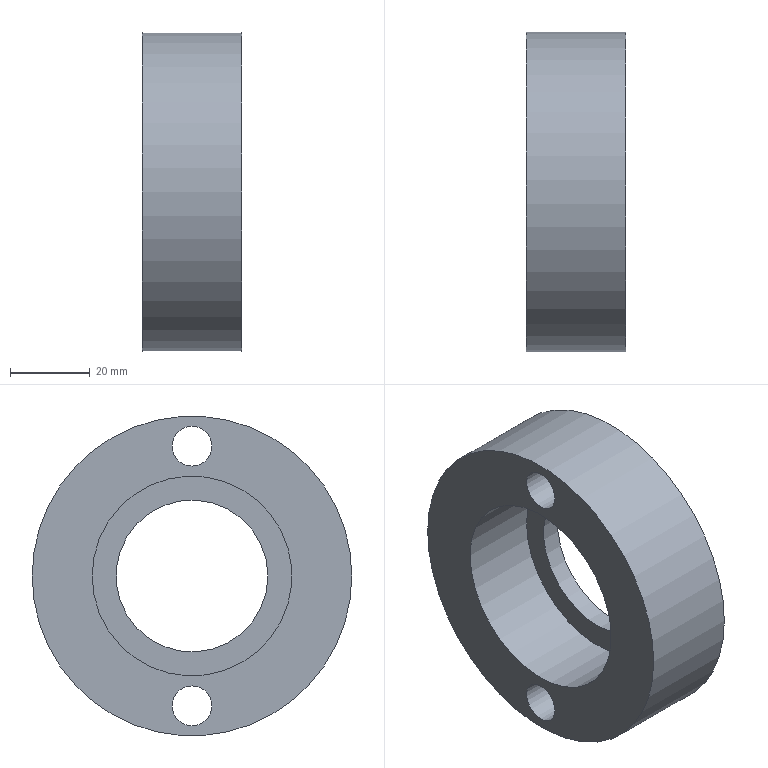Part | NX | features Hydraulic support1 2 | 1 solid | 8 faces | box 25 x 80 x 80 mm | volume 76796 mm3 | cylinder 5 | plane 3 | commonest cylinder face diameters 10 x2 38 x1 50 x1 80 x1
STEP:
#1=CARTESIAN_POINT('',(10.65,25.,0.));
#2=VERTEX_POINT('',#1);
#3=CARTESIAN_POINT('',(10.65,0.,0.));
#4=DIRECTION('',(1.,0.,0.));
#5=DIRECTION('',(0.,1.,0.));
#6=AXIS2_PLACEMENT_3D('',#3,#4,#5);
#7=CIRCLE('',#6,25.);
#8=EDGE_CURVE('',#2,#2,#7,.T.);
#9=ORIENTED_EDGE('',*,*,#8,.T.);
#10=EDGE_LOOP('',(#9));
#11=FACE_BOUND('',#10,.T.);
#12=CARTESIAN_POINT('',(-9.35,25.,0.));
#13=VERTEX_POINT('',#12);
#14=CARTESIAN_POINT('',(-9.35,0.,0.));
#15=DIRECTION('',(1.,0.,0.));
#16=DIRECTION('',(0.,1.,0.));
#17=AXIS2_PLACEMENT_3D('',#14,#15,#16);
#18=CIRCLE('',#17,25.);
#19=EDGE_CURVE('',#13,#13,#18,.F.);
#20=ORIENTED_EDGE('',*,*,#19,.T.);
#21=EDGE_LOOP('',(#20));
#22=FACE_BOUND('',#21,.T.);
#23=CARTESIAN_POINT('',(-9.35,0.,0.));
#24=DIRECTION('',(1.,0.,0.));
#25=DIRECTION('',(0.,1.,0.));
#26=AXIS2_PLACEMENT_3D('',#23,#24,#25);
#27=CYLINDRICAL_SURFACE('',#26,25.);
#28=ADVANCED_FACE('',(#11,#22),#27,.F.);
#29=CARTESIAN_POINT('',(-9.35,40.,0.));
#30=VERTEX_POINT('',#29);
#31=CARTESIAN_POINT('',(-9.35,0.,0.));
#32=DIRECTION('',(1.,0.,0.));
#33=DIRECTION('',(0.,1.,0.));
#34=AXIS2_PLACEMENT_3D('',#31,#32,#33);
#35=CIRCLE('',#34,40.);
#36=EDGE_CURVE('',#30,#30,#35,.T.);
#37=ORIENTED_EDGE('',*,*,#36,.F.);
#38=EDGE_LOOP('',(#37));
#39=FACE_BOUND('',#38,.T.);
#40=ORIENTED_EDGE('',*,*,#19,.F.);
#41=EDGE_LOOP('',(#40));
#42=FACE_BOUND('',#41,.T.);
#43=CARTESIAN_POINT('',(-9.35,0.,-37.5));
#44=VERTEX_POINT('',#43);
#45=CARTESIAN_POINT('',(-9.35,0.,-32.5));
#46=DIRECTION('',(1.,0.,0.));
#47=DIRECTION('',(0.,0.,-1.));
#48=AXIS2_PLACEMENT_3D('',#45,#46,#47);
#49=CIRCLE('',#48,5.);
#50=EDGE_CURVE('',#44,#44,#49,.T.);
#51=ORIENTED_EDGE('',*,*,#50,.T.);
#52=EDGE_LOOP('',(#51));
#53=FACE_BOUND('',#52,.T.);
#54=CARTESIAN_POINT('',(-9.35,0.,27.5));
#55=VERTEX_POINT('',#54);
#56=CARTESIAN_POINT('',(-9.35,0.,32.5));
#57=DIRECTION('',(1.,0.,0.));
#58=DIRECTION('',(0.,0.,-1.));
#59=AXIS2_PLACEMENT_3D('',#56,#57,#58);
#60=CIRCLE('',#59,5.);
#61=EDGE_CURVE('',#55,#55,#60,.T.);
#62=ORIENTED_EDGE('',*,*,#61,.T.);
#63=EDGE_LOOP('',(#62));
#64=FACE_BOUND('',#63,.T.);
#65=CARTESIAN_POINT('',(-9.35,0.,0.));
#66=DIRECTION('',(1.,0.,0.));
#67=DIRECTION('',(0.,1.,0.));
#68=AXIS2_PLACEMENT_3D('',#65,#66,#67);
#69=PLANE('',#68);
#70=ADVANCED_FACE('',(#39,#42,#53,#64),#69,.F.);
#71=ORIENTED_EDGE('',*,*,#8,.F.);
#72=EDGE_LOOP('',(#71));
#73=FACE_BOUND('',#72,.T.);
#74=CARTESIAN_POINT('',(10.65,-19.,0.));
#75=VERTEX_POINT('',#74);
#76=CARTESIAN_POINT('',(10.65,0.,0.));
#77=DIRECTION('',(-1.,0.,0.));
#78=DIRECTION('',(0.,-1.,0.));
#79=AXIS2_PLACEMENT_3D('',#76,#77,#78);
#80=CIRCLE('',#79,19.);
#81=EDGE_CURVE('',#75,#75,#80,.F.);
#82=ORIENTED_EDGE('',*,*,#81,.T.);
#83=EDGE_LOOP('',(#82));
#84=FACE_BOUND('',#83,.T.);
#85=CARTESIAN_POINT('',(10.65,0.,0.));
#86=DIRECTION('',(1.,0.,0.));
#87=DIRECTION('',(0.,1.,0.));
#88=AXIS2_PLACEMENT_3D('',#85,#86,#87);
#89=PLANE('',#88);
#90=ADVANCED_FACE('',(#73,#84),#89,.F.);
#91=CARTESIAN_POINT('',(15.65,0.,27.5));
#92=VERTEX_POINT('',#91);
#93=CARTESIAN_POINT('',(15.65,0.,32.5));
#94=DIRECTION('',(1.,0.,0.));
#95=DIRECTION('',(0.,0.,-1.));
#96=AXIS2_PLACEMENT_3D('',#93,#94,#95);
#97=CIRCLE('',#96,5.);
#98=EDGE_CURVE('',#92,#92,#97,.F.);
#99=ORIENTED_EDGE('',*,*,#98,.F.);
#100=EDGE_LOOP('',(#99));
#101=FACE_BOUND('',#100,.T.);
#102=ORIENTED_EDGE('',*,*,#61,.F.);
#103=EDGE_LOOP('',(#102));
#104=FACE_BOUND('',#103,.T.);
#105=CARTESIAN_POINT('',(15.65,0.,32.5));
#106=DIRECTION('',(1.,0.,0.));
#107=DIRECTION('',(0.,0.,-1.));
#108=AXIS2_PLACEMENT_3D('',#105,#106,#107);
#109=CYLINDRICAL_SURFACE('',#108,5.);
#110=ADVANCED_FACE('',(#101,#104),#109,.F.);
#111=CARTESIAN_POINT('',(15.65,0.,-37.5));
#112=VERTEX_POINT('',#111);
#113=CARTESIAN_POINT('',(15.65,0.,-32.5));
#114=DIRECTION('',(1.,0.,0.));
#115=DIRECTION('',(0.,0.,-1.));
#116=AXIS2_PLACEMENT_3D('',#113,#114,#115);
#117=CIRCLE('',#116,5.);
#118=EDGE_CURVE('',#112,#112,#117,.F.);
#119=ORIENTED_EDGE('',*,*,#118,.F.);
#120=EDGE_LOOP('',(#119));
#121=FACE_BOUND('',#120,.T.);
#122=ORIENTED_EDGE('',*,*,#50,.F.);
#123=EDGE_LOOP('',(#122));
#124=FACE_BOUND('',#123,.T.);
#125=CARTESIAN_POINT('',(15.65,0.,-32.5));
#126=DIRECTION('',(1.,0.,0.));
#127=DIRECTION('',(0.,0.,-1.));
#128=AXIS2_PLACEMENT_3D('',#125,#126,#127);
#129=CYLINDRICAL_SURFACE('',#128,5.);
#130=ADVANCED_FACE('',(#121,#124),#129,.F.);
#131=ORIENTED_EDGE('',*,*,#36,.T.);
#132=EDGE_LOOP('',(#131));
#133=FACE_BOUND('',#132,.T.);
#134=CARTESIAN_POINT('',(15.65,40.,0.));
#135=VERTEX_POINT('',#134);
#136=CARTESIAN_POINT('',(15.65,0.,0.));
#137=DIRECTION('',(1.,0.,0.));
#138=DIRECTION('',(0.,1.,0.));
#139=AXIS2_PLACEMENT_3D('',#136,#137,#138);
#140=CIRCLE('',#139,40.);
#141=EDGE_CURVE('',#135,#135,#140,.T.);
#142=ORIENTED_EDGE('',*,*,#141,.F.);
#143=EDGE_LOOP('',(#142));
#144=FACE_BOUND('',#143,.T.);
#145=CARTESIAN_POINT('',(-9.35,0.,0.));
#146=DIRECTION('',(1.,0.,0.));
#147=DIRECTION('',(0.,1.,0.));
#148=AXIS2_PLACEMENT_3D('',#145,#146,#147);
#149=CYLINDRICAL_SURFACE('',#148,40.);
#150=ADVANCED_FACE('',(#133,#144),#149,.T.);
#151=CARTESIAN_POINT('',(15.65,-19.,0.));
#152=VERTEX_POINT('',#151);
#153=CARTESIAN_POINT('',(15.65,0.,0.));
#154=DIRECTION('',(-1.,0.,0.));
#155=DIRECTION('',(0.,-1.,0.));
#156=AXIS2_PLACEMENT_3D('',#153,#154,#155);
#157=CIRCLE('',#156,19.);
#158=EDGE_CURVE('',#152,#152,#157,.T.);
#159=ORIENTED_EDGE('',*,*,#158,.F.);
#160=EDGE_LOOP('',(#159));
#161=FACE_BOUND('',#160,.T.);
#162=ORIENTED_EDGE('',*,*,#81,.F.);
#163=EDGE_LOOP('',(#162));
#164=FACE_BOUND('',#163,.T.);
#165=CARTESIAN_POINT('',(15.65,0.,0.));
#166=DIRECTION('',(-1.,0.,0.));
#167=DIRECTION('',(0.,-1.,0.));
#168=AXIS2_PLACEMENT_3D('',#165,#166,#167);
#169=CYLINDRICAL_SURFACE('',#168,19.);
#170=ADVANCED_FACE('',(#161,#164),#169,.F.);
#171=ORIENTED_EDGE('',*,*,#158,.T.);
#172=EDGE_LOOP('',(#171));
#173=FACE_BOUND('',#172,.T.);
#174=ORIENTED_EDGE('',*,*,#141,.T.);
#175=EDGE_LOOP('',(#174));
#176=FACE_BOUND('',#175,.T.);
#177=ORIENTED_EDGE('',*,*,#118,.T.);
#178=EDGE_LOOP('',(#177));
#179=FACE_BOUND('',#178,.T.);
#180=ORIENTED_EDGE('',*,*,#98,.T.);
#181=EDGE_LOOP('',(#180));
#182=FACE_BOUND('',#181,.T.);
#183=CARTESIAN_POINT('',(15.65,0.,0.));
#184=DIRECTION('',(1.,0.,0.));
#185=DIRECTION('',(0.,1.,0.));
#186=AXIS2_PLACEMENT_3D('',#183,#184,#185);
#187=PLANE('',#186);
#188=ADVANCED_FACE('',(#173,#176,#179,#182),#187,.T.);
#189=CLOSED_SHELL('',(#28,#70,#90,#110,#130,#150,#170,#188));
#190=MANIFOLD_SOLID_BREP('',#189);
#191=(LENGTH_UNIT()NAMED_UNIT(*)SI_UNIT(.MILLI.,.METRE.));
#192=UNCERTAINTY_MEASURE_WITH_UNIT(LENGTH_MEASURE(0.00001),#191,'','');
#193=(NAMED_UNIT(*)PLANE_ANGLE_UNIT()SI_UNIT($,.RADIAN.));
#194=(NAMED_UNIT(*)SI_UNIT($,.STERADIAN.)SOLID_ANGLE_UNIT());
#195=(GEOMETRIC_REPRESENTATION_CONTEXT(3)GLOBAL_UNCERTAINTY_ASSIGNED_CONTEXT((#192))GLOBAL_UNIT_ASSIGNED_CONTEXT((#191,#193,#194))REPRESENTATION_CONTEXT('',''));
#196=ADVANCED_BREP_SHAPE_REPRESENTATION('',(#190),#195);